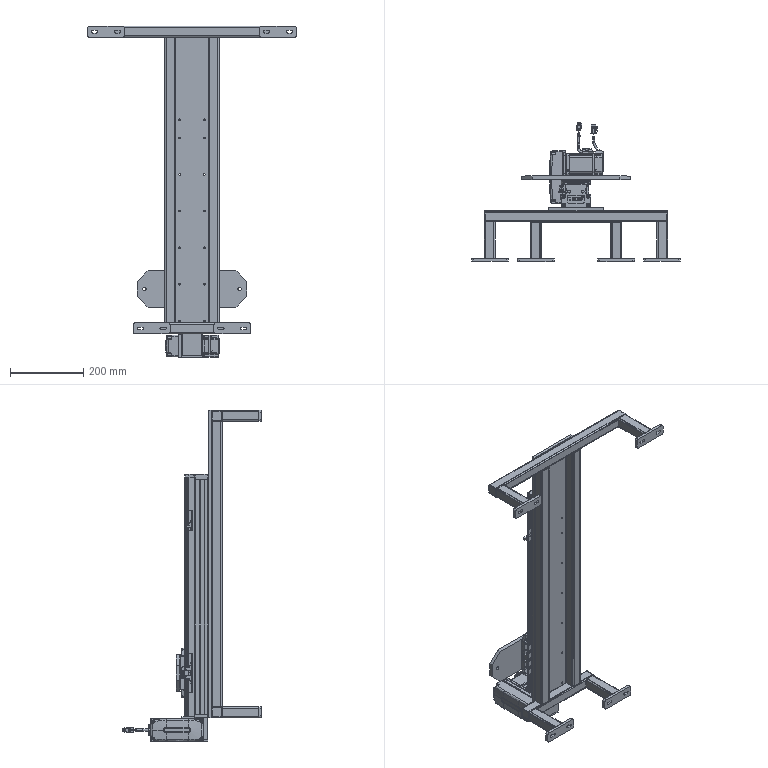Part | SolidWorks | features ReferencePattern 4, InContextFeatHolder 2, MirrorCompFeat 1 | 18 solids | 2237 faces | box 570 x 381.182 x 905.5 mm | volume 5879539 mm3 | plane 1078 | cylinder 901 | cone 134 | spline 83 | sphere 26 | torus 15 | commonest cylinder face diameters 1 x109 4 x88 8 x76 2 x63 3.3 x54 4.5 x46